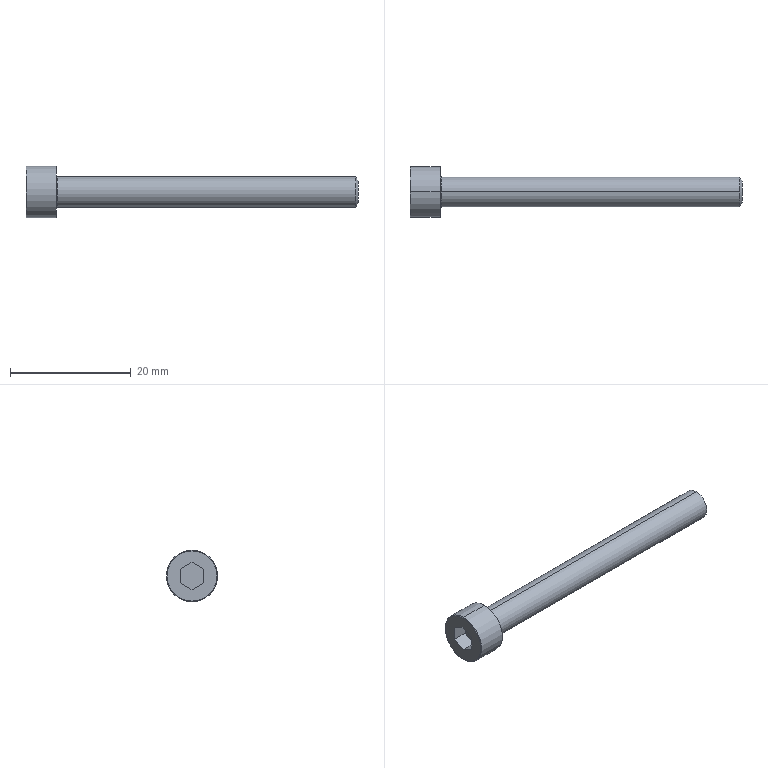Part | SolidWorks | features BaseBody 1 | 1 solid | 20 faces | box 55 x 8.5 x 8.5 mm | volume 1230 mm3 | plane 10 | torus 4 | cylinder 4 | cone 2 | commonest cylinder face diameters 5 x2 8.5 x2
STEP:
#1=CARTESIAN_POINT('',(0.,0.,4.15));
#2=VERTEX_POINT('',#1);
#3=CARTESIAN_POINT('',(0.,0.,-4.15));
#4=VERTEX_POINT('',#3);
#5=CARTESIAN_POINT('',(0.,0.,0.));
#6=DIRECTION('',(-1.,0.,0.));
#7=DIRECTION('',(0.,0.,-1.));
#8=AXIS2_PLACEMENT_3D('',#5,#6,#7);
#9=CIRCLE('',#8,4.15);
#10=EDGE_CURVE('',#2,#4,#9,.T.);
#11=ORIENTED_EDGE('',*,*,#10,.F.);
#12=CARTESIAN_POINT('',(0.1,0.,4.25));
#13=VERTEX_POINT('',#12);
#14=CARTESIAN_POINT('',(0.1,0.,4.15));
#15=DIRECTION('',(0.,1.,0.));
#16=DIRECTION('',(0.,0.,1.));
#17=AXIS2_PLACEMENT_3D('',#14,#15,#16);
#18=CIRCLE('',#17,0.1);
#19=EDGE_CURVE('',#2,#13,#18,.T.);
#20=ORIENTED_EDGE('',*,*,#19,.T.);
#21=CARTESIAN_POINT('',(0.1,0.,-4.25));
#22=VERTEX_POINT('',#21);
#23=CARTESIAN_POINT('',(0.1,0.,0.));
#24=DIRECTION('',(1.,0.,0.));
#25=DIRECTION('',(0.,0.,-1.));
#26=AXIS2_PLACEMENT_3D('',#23,#24,#25);
#27=CIRCLE('',#26,4.25);
#28=EDGE_CURVE('',#22,#13,#27,.T.);
#29=ORIENTED_EDGE('',*,*,#28,.F.);
#30=CARTESIAN_POINT('',(0.1,0.,-4.15));
#31=DIRECTION('',(0.,-1.,0.));
#32=DIRECTION('',(0.,0.,-1.));
#33=AXIS2_PLACEMENT_3D('',#30,#31,#32);
#34=CIRCLE('',#33,0.1);
#35=EDGE_CURVE('',#4,#22,#34,.T.);
#36=ORIENTED_EDGE('',*,*,#35,.F.);
#37=EDGE_LOOP('',(#11,#20,#29,#36));
#38=FACE_OUTER_BOUND('',#37,.T.);
#39=CARTESIAN_POINT('',(0.1,0.,0.));
#40=DIRECTION('',(1.,0.,0.));
#41=DIRECTION('',(0.,0.,-1.));
#42=AXIS2_PLACEMENT_3D('',#39,#40,#41);
#43=TOROIDAL_SURFACE('',#42,4.15,0.1);
#44=ADVANCED_FACE('',(#38),#43,.T.);
#45=CARTESIAN_POINT('',(55.,0.,1.807));
#46=VERTEX_POINT('',#45);
#47=CARTESIAN_POINT('',(55.,0.,-1.807));
#48=VERTEX_POINT('',#47);
#49=CARTESIAN_POINT('',(55.,0.,0.));
#50=DIRECTION('',(-1.,0.,0.));
#51=DIRECTION('',(0.,0.,1.));
#52=AXIS2_PLACEMENT_3D('',#49,#50,#51);
#53=CIRCLE('',#52,1.807);
#54=EDGE_CURVE('',#46,#48,#53,.T.);
#55=ORIENTED_EDGE('',*,*,#54,.T.);
#56=CARTESIAN_POINT('',(54.6,0.,-2.5));
#57=VERTEX_POINT('',#56);
#58=CARTESIAN_POINT('',(54.6,0.,-2.5));
#59=DIRECTION('',(-0.5,0.,-0.866));
#60=VECTOR('',#59,1000.);
#61=LINE('',#58,#60);
#62=EDGE_CURVE('',#48,#57,#61,.T.);
#63=ORIENTED_EDGE('',*,*,#62,.T.);
#64=CARTESIAN_POINT('',(54.6,0.,2.5));
#65=VERTEX_POINT('',#64);
#66=CARTESIAN_POINT('',(54.6,0.,0.));
#67=DIRECTION('',(-1.,0.,0.));
#68=DIRECTION('',(0.,0.,1.));
#69=AXIS2_PLACEMENT_3D('',#66,#67,#68);
#70=CIRCLE('',#69,2.5);
#71=EDGE_CURVE('',#65,#57,#70,.T.);
#72=ORIENTED_EDGE('',*,*,#71,.F.);
#73=CARTESIAN_POINT('',(54.6,0.,2.5));
#74=DIRECTION('',(-0.5,0.,0.866));
#75=VECTOR('',#74,1000.);
#76=LINE('',#73,#75);
#77=EDGE_CURVE('',#46,#65,#76,.T.);
#78=ORIENTED_EDGE('',*,*,#77,.F.);
#79=EDGE_LOOP('',(#55,#63,#72,#78));
#80=FACE_OUTER_BOUND('',#79,.T.);
#81=CARTESIAN_POINT('',(54.6,0.,0.));
#82=DIRECTION('',(-1.,0.,0.));
#83=DIRECTION('',(0.,0.,1.));
#84=AXIS2_PLACEMENT_3D('',#81,#82,#83);
#85=CONICAL_SURFACE('',#84,2.5,1.047);
#86=ADVANCED_FACE('',(#80),#85,.T.);
#87=CARTESIAN_POINT('',(5.,0.,-2.7));
#88=VERTEX_POINT('',#87);
#89=CARTESIAN_POINT('',(5.,0.,2.7));
#90=VERTEX_POINT('',#89);
#91=CARTESIAN_POINT('',(5.,0.,0.));
#92=DIRECTION('',(-1.,0.,0.));
#93=DIRECTION('',(0.,0.,1.));
#94=AXIS2_PLACEMENT_3D('',#91,#92,#93);
#95=CIRCLE('',#94,2.7);
#96=EDGE_CURVE('',#88,#90,#95,.T.);
#97=ORIENTED_EDGE('',*,*,#96,.F.);
#98=CARTESIAN_POINT('',(5.2,0.,-2.5));
#99=VERTEX_POINT('',#98);
#100=CARTESIAN_POINT('',(5.2,0.,-2.7));
#101=DIRECTION('',(0.,1.,0.));
#102=DIRECTION('',(0.,0.,1.));
#103=AXIS2_PLACEMENT_3D('',#100,#101,#102);
#104=CIRCLE('',#103,0.2);
#105=EDGE_CURVE('',#88,#99,#104,.T.);
#106=ORIENTED_EDGE('',*,*,#105,.T.);
#107=CARTESIAN_POINT('',(5.2,0.,2.5));
#108=VERTEX_POINT('',#107);
#109=CARTESIAN_POINT('',(5.2,0.,0.));
#110=DIRECTION('',(-1.,0.,0.));
#111=DIRECTION('',(0.,0.,1.));
#112=AXIS2_PLACEMENT_3D('',#109,#110,#111);
#113=CIRCLE('',#112,2.5);
#114=EDGE_CURVE('',#99,#108,#113,.T.);
#115=ORIENTED_EDGE('',*,*,#114,.T.);
#116=CARTESIAN_POINT('',(5.2,0.,2.7));
#117=DIRECTION('',(0.,-1.,0.));
#118=DIRECTION('',(0.,0.,-1.));
#119=AXIS2_PLACEMENT_3D('',#116,#117,#118);
#120=CIRCLE('',#119,0.2);
#121=EDGE_CURVE('',#90,#108,#120,.T.);
#122=ORIENTED_EDGE('',*,*,#121,.F.);
#123=EDGE_LOOP('',(#97,#106,#115,#122));
#124=FACE_OUTER_BOUND('',#123,.T.);
#125=CARTESIAN_POINT('',(5.2,0.,0.));
#126=DIRECTION('',(-1.,0.,0.));
#127=DIRECTION('',(0.,0.,1.));
#128=AXIS2_PLACEMENT_3D('',#125,#126,#127);
#129=TOROIDAL_SURFACE('',#128,2.7,0.2);
#130=ADVANCED_FACE('',(#124),#129,.F.);
#131=CARTESIAN_POINT('',(5.,0.,4.25));
#132=VERTEX_POINT('',#131);
#133=CARTESIAN_POINT('',(5.,0.,-4.25));
#134=VERTEX_POINT('',#133);
#135=CARTESIAN_POINT('',(5.,0.,0.));
#136=DIRECTION('',(-1.,0.,0.));
#137=DIRECTION('',(0.,0.,1.));
#138=AXIS2_PLACEMENT_3D('',#135,#136,#137);
#139=CIRCLE('',#138,4.25);
#140=EDGE_CURVE('',#132,#134,#139,.T.);
#141=ORIENTED_EDGE('',*,*,#140,.T.);
#142=CARTESIAN_POINT('',(0.,0.,-4.25));
#143=DIRECTION('',(-1.,0.,0.));
#144=VECTOR('',#143,1000.);
#145=LINE('',#142,#144);
#146=EDGE_CURVE('',#134,#22,#145,.T.);
#147=ORIENTED_EDGE('',*,*,#146,.T.);
#148=ORIENTED_EDGE('',*,*,#28,.T.);
#149=CARTESIAN_POINT('',(0.,0.,4.25));
#150=DIRECTION('',(-1.,0.,0.));
#151=VECTOR('',#150,1000.);
#152=LINE('',#149,#151);
#153=EDGE_CURVE('',#132,#13,#152,.T.);
#154=ORIENTED_EDGE('',*,*,#153,.F.);
#155=EDGE_LOOP('',(#141,#147,#148,#154));
#156=FACE_OUTER_BOUND('',#155,.T.);
#157=CARTESIAN_POINT('',(0.,0.,0.));
#158=DIRECTION('',(-1.,0.,0.));
#159=DIRECTION('',(0.,0.,1.));
#160=AXIS2_PLACEMENT_3D('',#157,#158,#159);
#161=CYLINDRICAL_SURFACE('',#160,4.25);
#162=ADVANCED_FACE('',(#156),#161,.T.);
#163=ORIENTED_EDGE('',*,*,#71,.T.);
#164=CARTESIAN_POINT('',(0.,0.,-2.5));
#165=DIRECTION('',(-1.,0.,0.));
#166=VECTOR('',#165,1000.);
#167=LINE('',#164,#166);
#168=EDGE_CURVE('',#57,#99,#167,.T.);
#169=ORIENTED_EDGE('',*,*,#168,.T.);
#170=CARTESIAN_POINT('',(5.2,0.,0.));
#171=DIRECTION('',(-1.,0.,0.));
#172=DIRECTION('',(0.,0.,1.));
#173=AXIS2_PLACEMENT_3D('',#170,#171,#172);
#174=CIRCLE('',#173,2.5);
#175=EDGE_CURVE('',#108,#99,#174,.T.);
#176=ORIENTED_EDGE('',*,*,#175,.F.);
#177=CARTESIAN_POINT('',(0.,0.,2.5));
#178=DIRECTION('',(-1.,0.,0.));
#179=VECTOR('',#178,1000.);
#180=LINE('',#177,#179);
#181=EDGE_CURVE('',#65,#108,#180,.T.);
#182=ORIENTED_EDGE('',*,*,#181,.F.);
#183=EDGE_LOOP('',(#163,#169,#176,#182));
#184=FACE_OUTER_BOUND('',#183,.T.);
#185=CARTESIAN_POINT('',(0.,0.,0.));
#186=DIRECTION('',(-1.,0.,0.));
#187=DIRECTION('',(0.,0.,1.));
#188=AXIS2_PLACEMENT_3D('',#185,#186,#187);
#189=CYLINDRICAL_SURFACE('',#188,2.5);
#190=ADVANCED_FACE('',(#184),#189,.T.);
#191=ORIENTED_EDGE('',*,*,#54,.F.);
#192=CARTESIAN_POINT('',(55.,0.,0.));
#193=DIRECTION('',(-1.,0.,0.));
#194=DIRECTION('',(0.,0.,1.));
#195=AXIS2_PLACEMENT_3D('',#192,#193,#194);
#196=CIRCLE('',#195,1.807);
#197=EDGE_CURVE('',#48,#46,#196,.T.);
#198=ORIENTED_EDGE('',*,*,#197,.F.);
#199=EDGE_LOOP('',(#191,#198));
#200=FACE_OUTER_BOUND('',#199,.T.);
#201=CARTESIAN_POINT('',(55.,2.5,0.));
#202=DIRECTION('',(-1.,0.,0.));
#203=DIRECTION('',(0.,0.,1.));
#204=AXIS2_PLACEMENT_3D('',#201,#202,#203);
#205=PLANE('',#204);
#206=ADVANCED_FACE('',(#200),#205,.F.);
#207=CARTESIAN_POINT('',(2.5,-1.983,1.145));
#208=VERTEX_POINT('',#207);
#209=CARTESIAN_POINT('',(2.5,0.,2.29));
#210=VERTEX_POINT('',#209);
#211=CARTESIAN_POINT('',(2.5,-1.983,1.145));
#212=DIRECTION('',(0.,0.866,0.5));
#213=VECTOR('',#212,1000.);
#214=LINE('',#211,#213);
#215=EDGE_CURVE('',#208,#210,#214,.T.);
#216=ORIENTED_EDGE('',*,*,#215,.T.);
#217=CARTESIAN_POINT('',(2.5,1.983,1.145));
#218=VERTEX_POINT('',#217);
#219=CARTESIAN_POINT('',(2.5,0.,2.29));
#220=DIRECTION('',(0.,0.866,-0.5));
#221=VECTOR('',#220,1000.);
#222=LINE('',#219,#221);
#223=EDGE_CURVE('',#210,#218,#222,.T.);
#224=ORIENTED_EDGE('',*,*,#223,.T.);
#225=CARTESIAN_POINT('',(2.5,1.983,-1.145));
#226=VERTEX_POINT('',#225);
#227=CARTESIAN_POINT('',(2.5,1.983,1.145));
#228=DIRECTION('',(0.,0.,-1.));
#229=VECTOR('',#228,1000.);
#230=LINE('',#227,#229);
#231=EDGE_CURVE('',#218,#226,#230,.T.);
#232=ORIENTED_EDGE('',*,*,#231,.T.);
#233=CARTESIAN_POINT('',(2.5,0.,-2.29));
#234=VERTEX_POINT('',#233);
#235=CARTESIAN_POINT('',(2.5,1.983,-1.145));
#236=DIRECTION('',(0.,-0.866,-0.5));
#237=VECTOR('',#236,1000.);
#238=LINE('',#235,#237);
#239=EDGE_CURVE('',#226,#234,#238,.T.);
#240=ORIENTED_EDGE('',*,*,#239,.T.);
#241=CARTESIAN_POINT('',(2.5,-1.983,-1.145));
#242=VERTEX_POINT('',#241);
#243=CARTESIAN_POINT('',(2.5,0.,-2.29));
#244=DIRECTION('',(0.,-0.866,0.5));
#245=VECTOR('',#244,1000.);
#246=LINE('',#243,#245);
#247=EDGE_CURVE('',#234,#242,#246,.T.);
#248=ORIENTED_EDGE('',*,*,#247,.T.);
#249=CARTESIAN_POINT('',(2.5,-1.983,-1.145));
#250=DIRECTION('',(0.,0.,1.));
#251=VECTOR('',#250,1000.);
#252=LINE('',#249,#251);
#253=EDGE_CURVE('',#242,#208,#252,.T.);
#254=ORIENTED_EDGE('',*,*,#253,.T.);
#255=EDGE_LOOP('',(#216,#224,#232,#240,#248,#254));
#256=FACE_OUTER_BOUND('',#255,.T.);
#257=CARTESIAN_POINT('',(2.5,-1.983,1.145));
#258=DIRECTION('',(1.,0.,0.));
#259=DIRECTION('',(0.,1.,0.));
#260=AXIS2_PLACEMENT_3D('',#257,#258,#259);
#261=PLANE('',#260);
#262=ADVANCED_FACE('',(#256),#261,.F.);
#263=CARTESIAN_POINT('',(0.,0.,2.29));
#264=VERTEX_POINT('',#263);
#265=CARTESIAN_POINT('',(0.,1.983,1.145));
#266=VERTEX_POINT('',#265);
#267=CARTESIAN_POINT('',(0.,0.,2.29));
#268=DIRECTION('',(0.,0.866,-0.5));
#269=VECTOR('',#268,1000.);
#270=LINE('',#267,#269);
#271=EDGE_CURVE('',#264,#266,#270,.T.);
#272=ORIENTED_EDGE('',*,*,#271,.T.);
#273=CARTESIAN_POINT('',(2.5,1.983,1.145));
#274=DIRECTION('',(-1.,0.,0.));
#275=VECTOR('',#274,1000.);
#276=LINE('',#273,#275);
#277=EDGE_CURVE('',#218,#266,#276,.T.);
#278=ORIENTED_EDGE('',*,*,#277,.F.);
#279=ORIENTED_EDGE('',*,*,#223,.F.);
#280=CARTESIAN_POINT('',(2.5,0.,2.29));
#281=DIRECTION('',(-1.,0.,0.));
#282=VECTOR('',#281,1000.);
#283=LINE('',#280,#282);
#284=EDGE_CURVE('',#210,#264,#283,.T.);
#285=ORIENTED_EDGE('',*,*,#284,.T.);
#286=EDGE_LOOP('',(#272,#278,#279,#285));
#287=FACE_OUTER_BOUND('',#286,.T.);
#288=CARTESIAN_POINT('',(2.5,0.,2.29));
#289=DIRECTION('',(0.,0.5,0.866));
#290=DIRECTION('',(1.,0.,0.));
#291=AXIS2_PLACEMENT_3D('',#288,#289,#290);
#292=PLANE('',#291);
#293=ADVANCED_FACE('',(#287),#292,.F.);
#294=CARTESIAN_POINT('',(0.,1.983,-1.145));
#295=VERTEX_POINT('',#294);
#296=CARTESIAN_POINT('',(0.,1.983,1.145));
#297=DIRECTION('',(0.,0.,-1.));
#298=VECTOR('',#297,1000.);
#299=LINE('',#296,#298);
#300=EDGE_CURVE('',#266,#295,#299,.T.);
#301=ORIENTED_EDGE('',*,*,#300,.T.);
#302=CARTESIAN_POINT('',(2.5,1.983,-1.145));
#303=DIRECTION('',(-1.,0.,0.));
#304=VECTOR('',#303,1000.);
#305=LINE('',#302,#304);
#306=EDGE_CURVE('',#226,#295,#305,.T.);
#307=ORIENTED_EDGE('',*,*,#306,.F.);
#308=ORIENTED_EDGE('',*,*,#231,.F.);
#309=ORIENTED_EDGE('',*,*,#277,.T.);
#310=EDGE_LOOP('',(#301,#307,#308,#309));
#311=FACE_OUTER_BOUND('',#310,.T.);
#312=CARTESIAN_POINT('',(2.5,1.983,1.145));
#313=DIRECTION('',(0.,1.,0.));
#314=DIRECTION('',(0.,0.,-1.));
#315=AXIS2_PLACEMENT_3D('',#312,#313,#314);
#316=PLANE('',#315);
#317=ADVANCED_FACE('',(#311),#316,.F.);
#318=CARTESIAN_POINT('',(0.,0.,-2.29));
#319=VERTEX_POINT('',#318);
#320=CARTESIAN_POINT('',(0.,1.983,-1.145));
#321=DIRECTION('',(0.,-0.866,-0.5));
#322=VECTOR('',#321,1000.);
#323=LINE('',#320,#322);
#324=EDGE_CURVE('',#295,#319,#323,.T.);
#325=ORIENTED_EDGE('',*,*,#324,.T.);
#326=CARTESIAN_POINT('',(2.5,0.,-2.29));
#327=DIRECTION('',(-1.,0.,0.));
#328=VECTOR('',#327,1000.);
#329=LINE('',#326,#328);
#330=EDGE_CURVE('',#234,#319,#329,.T.);
#331=ORIENTED_EDGE('',*,*,#330,.F.);
#332=ORIENTED_EDGE('',*,*,#239,.F.);
#333=ORIENTED_EDGE('',*,*,#306,.T.);
#334=EDGE_LOOP('',(#325,#331,#332,#333));
#335=FACE_OUTER_BOUND('',#334,.T.);
#336=CARTESIAN_POINT('',(2.5,1.983,-1.145));
#337=DIRECTION('',(0.,0.5,-0.866));
#338=DIRECTION('',(-1.,0.,0.));
#339=AXIS2_PLACEMENT_3D('',#336,#337,#338);
#340=PLANE('',#339);
#341=ADVANCED_FACE('',(#335),#340,.F.);
#342=CARTESIAN_POINT('',(0.,-1.983,-1.145));
#343=VERTEX_POINT('',#342);
#344=CARTESIAN_POINT('',(0.,0.,-2.29));
#345=DIRECTION('',(0.,-0.866,0.5));
#346=VECTOR('',#345,1000.);
#347=LINE('',#344,#346);
#348=EDGE_CURVE('',#319,#343,#347,.T.);
#349=ORIENTED_EDGE('',*,*,#348,.T.);
#350=CARTESIAN_POINT('',(2.5,-1.983,-1.145));
#351=DIRECTION('',(-1.,0.,0.));
#352=VECTOR('',#351,1000.);
#353=LINE('',#350,#352);
#354=EDGE_CURVE('',#242,#343,#353,.T.);
#355=ORIENTED_EDGE('',*,*,#354,.F.);
#356=ORIENTED_EDGE('',*,*,#247,.F.);
#357=ORIENTED_EDGE('',*,*,#330,.T.);
#358=EDGE_LOOP('',(#349,#355,#356,#357));
#359=FACE_OUTER_BOUND('',#358,.T.);
#360=CARTESIAN_POINT('',(2.5,0.,-2.29));
#361=DIRECTION('',(0.,-0.5,-0.866));
#362=DIRECTION('',(0.,-0.866,0.5));
#363=AXIS2_PLACEMENT_3D('',#360,#361,#362);
#364=PLANE('',#363);
#365=ADVANCED_FACE('',(#359),#364,.F.);
#366=CARTESIAN_POINT('',(0.,-1.983,1.145));
#367=VERTEX_POINT('',#366);
#368=CARTESIAN_POINT('',(0.,-1.983,-1.145));
#369=DIRECTION('',(0.,0.,1.));
#370=VECTOR('',#369,1000.);
#371=LINE('',#368,#370);
#372=EDGE_CURVE('',#343,#367,#371,.T.);
#373=ORIENTED_EDGE('',*,*,#372,.T.);
#374=CARTESIAN_POINT('',(2.5,-1.983,1.145));
#375=DIRECTION('',(-1.,0.,0.));
#376=VECTOR('',#375,1000.);
#377=LINE('',#374,#376);
#378=EDGE_CURVE('',#208,#367,#377,.T.);
#379=ORIENTED_EDGE('',*,*,#378,.F.);
#380=ORIENTED_EDGE('',*,*,#253,.F.);
#381=ORIENTED_EDGE('',*,*,#354,.T.);
#382=EDGE_LOOP('',(#373,#379,#380,#381));
#383=FACE_OUTER_BOUND('',#382,.T.);
#384=CARTESIAN_POINT('',(2.5,-1.983,-1.145));
#385=DIRECTION('',(0.,-1.,0.));
#386=DIRECTION('',(0.,0.,-1.));
#387=AXIS2_PLACEMENT_3D('',#384,#385,#386);
#388=PLANE('',#387);
#389=ADVANCED_FACE('',(#383),#388,.F.);
#390=CARTESIAN_POINT('',(0.,-1.983,1.145));
#391=DIRECTION('',(0.,0.866,0.5));
#392=VECTOR('',#391,1000.);
#393=LINE('',#390,#392);
#394=EDGE_CURVE('',#367,#264,#393,.T.);
#395=ORIENTED_EDGE('',*,*,#394,.T.);
#396=ORIENTED_EDGE('',*,*,#284,.F.);
#397=ORIENTED_EDGE('',*,*,#215,.F.);
#398=ORIENTED_EDGE('',*,*,#378,.T.);
#399=EDGE_LOOP('',(#395,#396,#397,#398));
#400=FACE_OUTER_BOUND('',#399,.T.);
#401=CARTESIAN_POINT('',(2.5,-1.983,1.145));
#402=DIRECTION('',(0.,-0.5,0.866));
#403=DIRECTION('',(-1.,0.,0.));
#404=AXIS2_PLACEMENT_3D('',#401,#402,#403);
#405=PLANE('',#404);
#406=ADVANCED_FACE('',(#400),#405,.F.);
#407=CARTESIAN_POINT('',(5.,0.,0.));
#408=DIRECTION('',(-1.,0.,0.));
#409=DIRECTION('',(0.,0.,1.));
#410=AXIS2_PLACEMENT_3D('',#407,#408,#409);
#411=CIRCLE('',#410,2.7);
#412=EDGE_CURVE('',#90,#88,#411,.T.);
#413=ORIENTED_EDGE('',*,*,#412,.T.);
#414=ORIENTED_EDGE('',*,*,#96,.T.);
#415=EDGE_LOOP('',(#413,#414));
#416=FACE_BOUND('',#415,.T.);
#417=ORIENTED_EDGE('',*,*,#140,.F.);
#418=CARTESIAN_POINT('',(5.,0.,0.));
#419=DIRECTION('',(-1.,0.,0.));
#420=DIRECTION('',(0.,0.,1.));
#421=AXIS2_PLACEMENT_3D('',#418,#419,#420);
#422=CIRCLE('',#421,4.25);
#423=EDGE_CURVE('',#134,#132,#422,.T.);
#424=ORIENTED_EDGE('',*,*,#423,.F.);
#425=EDGE_LOOP('',(#417,#424));
#426=FACE_OUTER_BOUND('',#425,.T.);
#427=CARTESIAN_POINT('',(5.,4.25,0.));
#428=DIRECTION('',(-1.,0.,0.));
#429=DIRECTION('',(0.,0.,1.));
#430=AXIS2_PLACEMENT_3D('',#427,#428,#429);
#431=PLANE('',#430);
#432=ADVANCED_FACE('',(#416,#426),#431,.F.);
#433=ORIENTED_EDGE('',*,*,#271,.F.);
#434=ORIENTED_EDGE('',*,*,#394,.F.);
#435=ORIENTED_EDGE('',*,*,#372,.F.);
#436=ORIENTED_EDGE('',*,*,#348,.F.);
#437=ORIENTED_EDGE('',*,*,#324,.F.);
#438=ORIENTED_EDGE('',*,*,#300,.F.);
#439=EDGE_LOOP('',(#433,#434,#435,#436,#437,#438));
#440=FACE_BOUND('',#439,.T.);
#441=CARTESIAN_POINT('',(0.,0.,0.));
#442=DIRECTION('',(-1.,0.,0.));
#443=DIRECTION('',(0.,0.,-1.));
#444=AXIS2_PLACEMENT_3D('',#441,#442,#443);
#445=CIRCLE('',#444,4.15);
#446=EDGE_CURVE('',#4,#2,#445,.T.);
#447=ORIENTED_EDGE('',*,*,#446,.T.);
#448=ORIENTED_EDGE('',*,*,#10,.T.);
#449=EDGE_LOOP('',(#447,#448));
#450=FACE_OUTER_BOUND('',#449,.T.);
#451=CARTESIAN_POINT('',(0.,0.,0.));
#452=DIRECTION('',(1.,0.,0.));
#453=DIRECTION('',(0.,1.,0.));
#454=AXIS2_PLACEMENT_3D('',#451,#452,#453);
#455=PLANE('',#454);
#456=ADVANCED_FACE('',(#440,#450),#455,.F.);
#457=ORIENTED_EDGE('',*,*,#168,.F.);
#458=CARTESIAN_POINT('',(54.6,0.,0.));
#459=DIRECTION('',(-1.,0.,0.));
#460=DIRECTION('',(0.,0.,1.));
#461=AXIS2_PLACEMENT_3D('',#458,#459,#460);
#462=CIRCLE('',#461,2.5);
#463=EDGE_CURVE('',#57,#65,#462,.T.);
#464=ORIENTED_EDGE('',*,*,#463,.T.);
#465=ORIENTED_EDGE('',*,*,#181,.T.);
#466=ORIENTED_EDGE('',*,*,#114,.F.);
#467=EDGE_LOOP('',(#457,#464,#465,#466));
#468=FACE_OUTER_BOUND('',#467,.T.);
#469=CARTESIAN_POINT('',(0.,0.,0.));
#470=DIRECTION('',(-1.,0.,0.));
#471=DIRECTION('',(0.,0.,1.));
#472=AXIS2_PLACEMENT_3D('',#469,#470,#471);
#473=CYLINDRICAL_SURFACE('',#472,2.5);
#474=ADVANCED_FACE('',(#468),#473,.T.);
#475=ORIENTED_EDGE('',*,*,#146,.F.);
#476=ORIENTED_EDGE('',*,*,#423,.T.);
#477=ORIENTED_EDGE('',*,*,#153,.T.);
#478=CARTESIAN_POINT('',(0.1,0.,0.));
#479=DIRECTION('',(1.,0.,0.));
#480=DIRECTION('',(0.,0.,-1.));
#481=AXIS2_PLACEMENT_3D('',#478,#479,#480);
#482=CIRCLE('',#481,4.25);
#483=EDGE_CURVE('',#13,#22,#482,.T.);
#484=ORIENTED_EDGE('',*,*,#483,.T.);
#485=EDGE_LOOP('',(#475,#476,#477,#484));
#486=FACE_OUTER_BOUND('',#485,.T.);
#487=CARTESIAN_POINT('',(0.,0.,0.));
#488=DIRECTION('',(-1.,0.,0.));
#489=DIRECTION('',(0.,0.,1.));
#490=AXIS2_PLACEMENT_3D('',#487,#488,#489);
#491=CYLINDRICAL_SURFACE('',#490,4.25);
#492=ADVANCED_FACE('',(#486),#491,.T.);
#493=ORIENTED_EDGE('',*,*,#105,.F.);
#494=ORIENTED_EDGE('',*,*,#412,.F.);
#495=ORIENTED_EDGE('',*,*,#121,.T.);
#496=ORIENTED_EDGE('',*,*,#175,.T.);
#497=EDGE_LOOP('',(#493,#494,#495,#496));
#498=FACE_OUTER_BOUND('',#497,.T.);
#499=CARTESIAN_POINT('',(5.2,0.,0.));
#500=DIRECTION('',(-1.,0.,0.));
#501=DIRECTION('',(0.,0.,1.));
#502=AXIS2_PLACEMENT_3D('',#499,#500,#501);
#503=TOROIDAL_SURFACE('',#502,2.7,0.2);
#504=ADVANCED_FACE('',(#498),#503,.F.);
#505=ORIENTED_EDGE('',*,*,#62,.F.);
#506=ORIENTED_EDGE('',*,*,#197,.T.);
#507=ORIENTED_EDGE('',*,*,#77,.T.);
#508=ORIENTED_EDGE('',*,*,#463,.F.);
#509=EDGE_LOOP('',(#505,#506,#507,#508));
#510=FACE_OUTER_BOUND('',#509,.T.);
#511=CARTESIAN_POINT('',(54.6,0.,0.));
#512=DIRECTION('',(-1.,0.,0.));
#513=DIRECTION('',(0.,0.,1.));
#514=AXIS2_PLACEMENT_3D('',#511,#512,#513);
#515=CONICAL_SURFACE('',#514,2.5,1.047);
#516=ADVANCED_FACE('',(#510),#515,.T.);
#517=ORIENTED_EDGE('',*,*,#19,.F.);
#518=ORIENTED_EDGE('',*,*,#446,.F.);
#519=ORIENTED_EDGE('',*,*,#35,.T.);
#520=ORIENTED_EDGE('',*,*,#483,.F.);
#521=EDGE_LOOP('',(#517,#518,#519,#520));
#522=FACE_OUTER_BOUND('',#521,.T.);
#523=CARTESIAN_POINT('',(0.1,0.,0.));
#524=DIRECTION('',(1.,0.,0.));
#525=DIRECTION('',(0.,0.,-1.));
#526=AXIS2_PLACEMENT_3D('',#523,#524,#525);
#527=TOROIDAL_SURFACE('',#526,4.15,0.1);
#528=ADVANCED_FACE('',(#522),#527,.T.);
#529=CLOSED_SHELL('',(#44,#86,#130,#162,#190,#206,#262,#293,#317,#341,#365,#389,#406,#432,#456,#474,#492,#504,#516,#528));
#530=MANIFOLD_SOLID_BREP('',#529);
#531=CARTESIAN_POINT('',(0.,0.,0.));
#532=DIRECTION('',(0.,0.,1.));
#533=DIRECTION('',(1.,0.,0.));
#534=AXIS2_PLACEMENT_3D('',#531,#532,#533);
#535=(LENGTH_UNIT()NAMED_UNIT(*)SI_UNIT(.MILLI.,.METRE.));
#536=UNCERTAINTY_MEASURE_WITH_UNIT(LENGTH_MEASURE(0.00001),#535,'','');
#537=(NAMED_UNIT(*)PLANE_ANGLE_UNIT()SI_UNIT($,.RADIAN.));
#538=(NAMED_UNIT(*)SI_UNIT($,.STERADIAN.)SOLID_ANGLE_UNIT());
#539=(GEOMETRIC_REPRESENTATION_CONTEXT(3)GLOBAL_UNCERTAINTY_ASSIGNED_CONTEXT((#536))GLOBAL_UNIT_ASSIGNED_CONTEXT((#535,#537,#538))REPRESENTATION_CONTEXT('',''));
#540=ADVANCED_BREP_SHAPE_REPRESENTATION('',(#530,#534),#539);